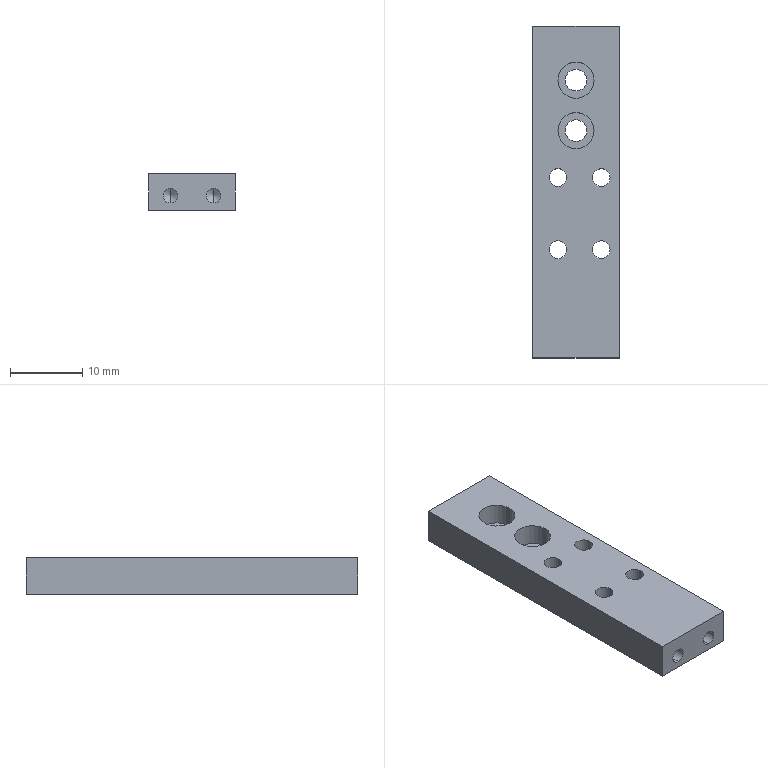Part | SolidWorks | features BaseBody 1 | 1 solid | 32 faces | box 12 x 46 x 5 mm | volume 2467 mm3 | cylinder 20 | plane 8 | cone 4 | commonest cylinder face diameters 2.459 x8 2.013 x4 3 x4 5 x4
STEP:
#1=CARTESIAN_POINT('',(2.595,24.168,0.));
#2=VERTEX_POINT('',#1);
#3=CARTESIAN_POINT('',(-0.4046,24.168,0.));
#4=VERTEX_POINT('',#3);
#5=CARTESIAN_POINT('',(1.095,24.168,0.));
#6=DIRECTION('',(0.,0.,-1.));
#7=DIRECTION('',(1.,0.,0.));
#8=AXIS2_PLACEMENT_3D('',#5,#6,#7);
#9=CIRCLE('',#8,1.5);
#10=EDGE_CURVE('',#2,#4,#9,.T.);
#11=ORIENTED_EDGE('',*,*,#10,.T.);
#12=CARTESIAN_POINT('',(-0.4046,24.168,2.));
#13=VERTEX_POINT('',#12);
#14=CARTESIAN_POINT('',(-0.4046,24.168,-42.802));
#15=DIRECTION('',(0.,0.,1.));
#16=VECTOR('',#15,1000.);
#17=LINE('',#14,#16);
#18=EDGE_CURVE('',#4,#13,#17,.T.);
#19=ORIENTED_EDGE('',*,*,#18,.T.);
#20=CARTESIAN_POINT('',(2.595,24.168,2.));
#21=VERTEX_POINT('',#20);
#22=CARTESIAN_POINT('',(1.095,24.168,2.));
#23=DIRECTION('',(0.,0.,-1.));
#24=DIRECTION('',(1.,0.,0.));
#25=AXIS2_PLACEMENT_3D('',#22,#23,#24);
#26=CIRCLE('',#25,1.5);
#27=EDGE_CURVE('',#21,#13,#26,.T.);
#28=ORIENTED_EDGE('',*,*,#27,.F.);
#29=CARTESIAN_POINT('',(2.595,24.168,-42.802));
#30=DIRECTION('',(0.,0.,1.));
#31=VECTOR('',#30,1000.);
#32=LINE('',#29,#31);
#33=EDGE_CURVE('',#2,#21,#32,.T.);
#34=ORIENTED_EDGE('',*,*,#33,.F.);
#35=EDGE_LOOP('',(#11,#19,#28,#34));
#36=FACE_OUTER_BOUND('',#35,.T.);
#37=CARTESIAN_POINT('',(1.095,24.168,-42.802));
#38=DIRECTION('',(0.,0.,1.));
#39=DIRECTION('',(1.,0.,0.));
#40=AXIS2_PLACEMENT_3D('',#37,#38,#39);
#41=CYLINDRICAL_SURFACE('',#40,1.5);
#42=ADVANCED_FACE('',(#36),#41,.F.);
#43=CARTESIAN_POINT('',(2.595,31.168,0.));
#44=VERTEX_POINT('',#43);
#45=CARTESIAN_POINT('',(-0.4046,31.168,0.));
#46=VERTEX_POINT('',#45);
#47=CARTESIAN_POINT('',(1.095,31.168,0.));
#48=DIRECTION('',(0.,0.,-1.));
#49=DIRECTION('',(1.,0.,0.));
#50=AXIS2_PLACEMENT_3D('',#47,#48,#49);
#51=CIRCLE('',#50,1.5);
#52=EDGE_CURVE('',#44,#46,#51,.T.);
#53=ORIENTED_EDGE('',*,*,#52,.T.);
#54=CARTESIAN_POINT('',(-0.4046,31.168,2.));
#55=VERTEX_POINT('',#54);
#56=CARTESIAN_POINT('',(-0.4046,31.168,-42.802));
#57=DIRECTION('',(0.,0.,1.));
#58=VECTOR('',#57,1000.);
#59=LINE('',#56,#58);
#60=EDGE_CURVE('',#46,#55,#59,.T.);
#61=ORIENTED_EDGE('',*,*,#60,.T.);
#62=CARTESIAN_POINT('',(2.595,31.168,2.));
#63=VERTEX_POINT('',#62);
#64=CARTESIAN_POINT('',(1.095,31.168,2.));
#65=DIRECTION('',(0.,0.,-1.));
#66=DIRECTION('',(1.,0.,0.));
#67=AXIS2_PLACEMENT_3D('',#64,#65,#66);
#68=CIRCLE('',#67,1.5);
#69=EDGE_CURVE('',#63,#55,#68,.T.);
#70=ORIENTED_EDGE('',*,*,#69,.F.);
#71=CARTESIAN_POINT('',(2.595,31.168,-42.802));
#72=DIRECTION('',(0.,0.,1.));
#73=VECTOR('',#72,1000.);
#74=LINE('',#71,#73);
#75=EDGE_CURVE('',#44,#63,#74,.T.);
#76=ORIENTED_EDGE('',*,*,#75,.F.);
#77=EDGE_LOOP('',(#53,#61,#70,#76));
#78=FACE_OUTER_BOUND('',#77,.T.);
#79=CARTESIAN_POINT('',(1.095,31.168,-42.802));
#80=DIRECTION('',(0.,0.,1.));
#81=DIRECTION('',(1.,0.,0.));
#82=AXIS2_PLACEMENT_3D('',#79,#80,#81);
#83=CYLINDRICAL_SURFACE('',#82,1.5);
#84=ADVANCED_FACE('',(#78),#83,.F.);
#85=CARTESIAN_POINT('',(-0.1751,7.668,0.));
#86=VERTEX_POINT('',#85);
#87=CARTESIAN_POINT('',(-2.634,7.668,0.));
#88=VERTEX_POINT('',#87);
#89=CARTESIAN_POINT('',(-1.405,7.668,0.));
#90=DIRECTION('',(0.,0.,-1.));
#91=DIRECTION('',(1.,0.,0.));
#92=AXIS2_PLACEMENT_3D('',#89,#90,#91);
#93=CIRCLE('',#92,1.23);
#94=EDGE_CURVE('',#86,#88,#93,.T.);
#95=ORIENTED_EDGE('',*,*,#94,.T.);
#96=CARTESIAN_POINT('',(-2.634,7.668,5.));
#97=VERTEX_POINT('',#96);
#98=CARTESIAN_POINT('',(-2.634,7.668,-42.802));
#99=DIRECTION('',(0.,0.,1.));
#100=VECTOR('',#99,1000.);
#101=LINE('',#98,#100);
#102=EDGE_CURVE('',#88,#97,#101,.T.);
#103=ORIENTED_EDGE('',*,*,#102,.T.);
#104=CARTESIAN_POINT('',(-0.1751,7.668,5.));
#105=VERTEX_POINT('',#104);
#106=CARTESIAN_POINT('',(-1.405,7.668,5.));
#107=DIRECTION('',(0.,0.,-1.));
#108=DIRECTION('',(1.,0.,0.));
#109=AXIS2_PLACEMENT_3D('',#106,#107,#108);
#110=CIRCLE('',#109,1.23);
#111=EDGE_CURVE('',#105,#97,#110,.T.);
#112=ORIENTED_EDGE('',*,*,#111,.F.);
#113=CARTESIAN_POINT('',(-0.1751,7.668,-42.802));
#114=DIRECTION('',(0.,0.,1.));
#115=VECTOR('',#114,1000.);
#116=LINE('',#113,#115);
#117=EDGE_CURVE('',#86,#105,#116,.T.);
#118=ORIENTED_EDGE('',*,*,#117,.F.);
#119=EDGE_LOOP('',(#95,#103,#112,#118));
#120=FACE_OUTER_BOUND('',#119,.T.);
#121=CARTESIAN_POINT('',(-1.405,7.668,-42.802));
#122=DIRECTION('',(0.,0.,1.));
#123=DIRECTION('',(1.,0.,0.));
#124=AXIS2_PLACEMENT_3D('',#121,#122,#123);
#125=CYLINDRICAL_SURFACE('',#124,1.23);
#126=ADVANCED_FACE('',(#120),#125,.F.);
#127=CARTESIAN_POINT('',(-0.1751,17.668,0.));
#128=VERTEX_POINT('',#127);
#129=CARTESIAN_POINT('',(-2.634,17.668,0.));
#130=VERTEX_POINT('',#129);
#131=CARTESIAN_POINT('',(-1.405,17.668,0.));
#132=DIRECTION('',(0.,0.,-1.));
#133=DIRECTION('',(1.,0.,0.));
#134=AXIS2_PLACEMENT_3D('',#131,#132,#133);
#135=CIRCLE('',#134,1.23);
#136=EDGE_CURVE('',#128,#130,#135,.T.);
#137=ORIENTED_EDGE('',*,*,#136,.T.);
#138=CARTESIAN_POINT('',(-2.634,17.668,5.));
#139=VERTEX_POINT('',#138);
#140=CARTESIAN_POINT('',(-2.634,17.668,-42.802));
#141=DIRECTION('',(0.,0.,1.));
#142=VECTOR('',#141,1000.);
#143=LINE('',#140,#142);
#144=EDGE_CURVE('',#130,#139,#143,.T.);
#145=ORIENTED_EDGE('',*,*,#144,.T.);
#146=CARTESIAN_POINT('',(-0.1751,17.668,5.));
#147=VERTEX_POINT('',#146);
#148=CARTESIAN_POINT('',(-1.405,17.668,5.));
#149=DIRECTION('',(0.,0.,-1.));
#150=DIRECTION('',(1.,0.,0.));
#151=AXIS2_PLACEMENT_3D('',#148,#149,#150);
#152=CIRCLE('',#151,1.23);
#153=EDGE_CURVE('',#147,#139,#152,.T.);
#154=ORIENTED_EDGE('',*,*,#153,.F.);
#155=CARTESIAN_POINT('',(-0.1751,17.668,-42.802));
#156=DIRECTION('',(0.,0.,1.));
#157=VECTOR('',#156,1000.);
#158=LINE('',#155,#157);
#159=EDGE_CURVE('',#128,#147,#158,.T.);
#160=ORIENTED_EDGE('',*,*,#159,.F.);
#161=EDGE_LOOP('',(#137,#145,#154,#160));
#162=FACE_OUTER_BOUND('',#161,.T.);
#163=CARTESIAN_POINT('',(-1.405,17.668,-42.802));
#164=DIRECTION('',(0.,0.,1.));
#165=DIRECTION('',(1.,0.,0.));
#166=AXIS2_PLACEMENT_3D('',#163,#164,#165);
#167=CYLINDRICAL_SURFACE('',#166,1.23);
#168=ADVANCED_FACE('',(#162),#167,.F.);
#169=CARTESIAN_POINT('',(5.825,17.668,0.));
#170=VERTEX_POINT('',#169);
#171=CARTESIAN_POINT('',(3.366,17.668,0.));
#172=VERTEX_POINT('',#171);
#173=CARTESIAN_POINT('',(4.595,17.668,0.));
#174=DIRECTION('',(0.,0.,-1.));
#175=DIRECTION('',(1.,0.,0.));
#176=AXIS2_PLACEMENT_3D('',#173,#174,#175);
#177=CIRCLE('',#176,1.229);
#178=EDGE_CURVE('',#170,#172,#177,.T.);
#179=ORIENTED_EDGE('',*,*,#178,.T.);
#180=CARTESIAN_POINT('',(3.366,17.668,5.));
#181=VERTEX_POINT('',#180);
#182=CARTESIAN_POINT('',(3.366,17.668,-42.802));
#183=DIRECTION('',(0.,0.,1.));
#184=VECTOR('',#183,1000.);
#185=LINE('',#182,#184);
#186=EDGE_CURVE('',#172,#181,#185,.T.);
#187=ORIENTED_EDGE('',*,*,#186,.T.);
#188=CARTESIAN_POINT('',(5.825,17.668,5.));
#189=VERTEX_POINT('',#188);
#190=CARTESIAN_POINT('',(4.595,17.668,5.));
#191=DIRECTION('',(0.,0.,-1.));
#192=DIRECTION('',(1.,0.,0.));
#193=AXIS2_PLACEMENT_3D('',#190,#191,#192);
#194=CIRCLE('',#193,1.229);
#195=EDGE_CURVE('',#189,#181,#194,.T.);
#196=ORIENTED_EDGE('',*,*,#195,.F.);
#197=CARTESIAN_POINT('',(5.825,17.668,-42.802));
#198=DIRECTION('',(0.,0.,1.));
#199=VECTOR('',#198,1000.);
#200=LINE('',#197,#199);
#201=EDGE_CURVE('',#170,#189,#200,.T.);
#202=ORIENTED_EDGE('',*,*,#201,.F.);
#203=EDGE_LOOP('',(#179,#187,#196,#202));
#204=FACE_OUTER_BOUND('',#203,.T.);
#205=CARTESIAN_POINT('',(4.595,17.668,-42.802));
#206=DIRECTION('',(0.,0.,1.));
#207=DIRECTION('',(1.,0.,0.));
#208=AXIS2_PLACEMENT_3D('',#205,#206,#207);
#209=CYLINDRICAL_SURFACE('',#208,1.229);
#210=ADVANCED_FACE('',(#204),#209,.F.);
#211=CARTESIAN_POINT('',(5.825,7.668,0.));
#212=VERTEX_POINT('',#211);
#213=CARTESIAN_POINT('',(3.366,7.668,0.));
#214=VERTEX_POINT('',#213);
#215=CARTESIAN_POINT('',(4.595,7.668,0.));
#216=DIRECTION('',(0.,0.,-1.));
#217=DIRECTION('',(1.,0.,0.));
#218=AXIS2_PLACEMENT_3D('',#215,#216,#217);
#219=CIRCLE('',#218,1.23);
#220=EDGE_CURVE('',#212,#214,#219,.T.);
#221=ORIENTED_EDGE('',*,*,#220,.T.);
#222=CARTESIAN_POINT('',(3.366,7.668,5.));
#223=VERTEX_POINT('',#222);
#224=CARTESIAN_POINT('',(3.366,7.668,-42.802));
#225=DIRECTION('',(0.,0.,1.));
#226=VECTOR('',#225,1000.);
#227=LINE('',#224,#226);
#228=EDGE_CURVE('',#214,#223,#227,.T.);
#229=ORIENTED_EDGE('',*,*,#228,.T.);
#230=CARTESIAN_POINT('',(5.825,7.668,5.));
#231=VERTEX_POINT('',#230);
#232=CARTESIAN_POINT('',(4.595,7.668,5.));
#233=DIRECTION('',(0.,0.,-1.));
#234=DIRECTION('',(1.,0.,0.));
#235=AXIS2_PLACEMENT_3D('',#232,#233,#234);
#236=CIRCLE('',#235,1.23);
#237=EDGE_CURVE('',#231,#223,#236,.T.);
#238=ORIENTED_EDGE('',*,*,#237,.F.);
#239=CARTESIAN_POINT('',(5.825,7.668,-42.802));
#240=DIRECTION('',(0.,0.,1.));
#241=VECTOR('',#240,1000.);
#242=LINE('',#239,#241);
#243=EDGE_CURVE('',#212,#231,#242,.T.);
#244=ORIENTED_EDGE('',*,*,#243,.F.);
#245=EDGE_LOOP('',(#221,#229,#238,#244));
#246=FACE_OUTER_BOUND('',#245,.T.);
#247=CARTESIAN_POINT('',(4.595,7.668,-42.802));
#248=DIRECTION('',(0.,0.,1.));
#249=DIRECTION('',(1.,0.,0.));
#250=AXIS2_PLACEMENT_3D('',#247,#248,#249);
#251=CYLINDRICAL_SURFACE('',#250,1.23);
#252=ADVANCED_FACE('',(#246),#251,.F.);
#253=CARTESIAN_POINT('',(-1.905,0.6681,3.006));
#254=VERTEX_POINT('',#253);
#255=CARTESIAN_POINT('',(-1.905,0.6681,0.9935));
#256=VERTEX_POINT('',#255);
#257=CARTESIAN_POINT('',(-1.905,0.6681,2.));
#258=DIRECTION('',(0.,-1.,0.));
#259=DIRECTION('',(0.,0.,-1.));
#260=AXIS2_PLACEMENT_3D('',#257,#258,#259);
#261=CIRCLE('',#260,1.006);
#262=EDGE_CURVE('',#254,#256,#261,.T.);
#263=ORIENTED_EDGE('',*,*,#262,.F.);
#264=CARTESIAN_POINT('',(-1.905,-7.332,3.006));
#265=VERTEX_POINT('',#264);
#266=CARTESIAN_POINT('',(-1.905,-3.332,3.006));
#267=DIRECTION('',(0.,-1.,0.));
#268=VECTOR('',#267,1000.);
#269=LINE('',#266,#268);
#270=EDGE_CURVE('',#254,#265,#269,.T.);
#271=ORIENTED_EDGE('',*,*,#270,.T.);
#272=CARTESIAN_POINT('',(-1.905,-7.332,0.9935));
#273=VERTEX_POINT('',#272);
#274=CARTESIAN_POINT('',(-1.905,-7.332,2.));
#275=DIRECTION('',(0.,1.,0.));
#276=DIRECTION('',(0.,0.,-1.));
#277=AXIS2_PLACEMENT_3D('',#274,#275,#276);
#278=CIRCLE('',#277,1.006);
#279=EDGE_CURVE('',#273,#265,#278,.T.);
#280=ORIENTED_EDGE('',*,*,#279,.F.);
#281=CARTESIAN_POINT('',(-1.905,-3.332,0.9935));
#282=DIRECTION('',(0.,-1.,0.));
#283=VECTOR('',#282,1000.);
#284=LINE('',#281,#283);
#285=EDGE_CURVE('',#256,#273,#284,.T.);
#286=ORIENTED_EDGE('',*,*,#285,.F.);
#287=EDGE_LOOP('',(#263,#271,#280,#286));
#288=FACE_OUTER_BOUND('',#287,.T.);
#289=CARTESIAN_POINT('',(-1.905,-3.332,2.));
#290=DIRECTION('',(0.,-1.,0.));
#291=DIRECTION('',(0.,0.,-1.));
#292=AXIS2_PLACEMENT_3D('',#289,#290,#291);
#293=CYLINDRICAL_SURFACE('',#292,1.006);
#294=ADVANCED_FACE('',(#288),#293,.F.);
#295=CARTESIAN_POINT('',(4.095,0.6681,3.006));
#296=VERTEX_POINT('',#295);
#297=CARTESIAN_POINT('',(4.095,0.6681,0.9935));
#298=VERTEX_POINT('',#297);
#299=CARTESIAN_POINT('',(4.095,0.6681,2.));
#300=DIRECTION('',(0.,-1.,0.));
#301=DIRECTION('',(0.,0.,-1.));
#302=AXIS2_PLACEMENT_3D('',#299,#300,#301);
#303=CIRCLE('',#302,1.006);
#304=EDGE_CURVE('',#296,#298,#303,.T.);
#305=ORIENTED_EDGE('',*,*,#304,.F.);
#306=CARTESIAN_POINT('',(4.095,-7.332,3.006));
#307=VERTEX_POINT('',#306);
#308=CARTESIAN_POINT('',(4.095,-3.332,3.006));
#309=DIRECTION('',(0.,-1.,0.));
#310=VECTOR('',#309,1000.);
#311=LINE('',#308,#310);
#312=EDGE_CURVE('',#296,#307,#311,.T.);
#313=ORIENTED_EDGE('',*,*,#312,.T.);
#314=CARTESIAN_POINT('',(4.095,-7.332,0.9935));
#315=VERTEX_POINT('',#314);
#316=CARTESIAN_POINT('',(4.095,-7.332,2.));
#317=DIRECTION('',(0.,1.,0.));
#318=DIRECTION('',(0.,0.,-1.));
#319=AXIS2_PLACEMENT_3D('',#316,#317,#318);
#320=CIRCLE('',#319,1.006);
#321=EDGE_CURVE('',#315,#307,#320,.T.);
#322=ORIENTED_EDGE('',*,*,#321,.F.);
#323=CARTESIAN_POINT('',(4.095,-3.332,0.9935));
#324=DIRECTION('',(0.,-1.,0.));
#325=VECTOR('',#324,1000.);
#326=LINE('',#323,#325);
#327=EDGE_CURVE('',#298,#315,#326,.T.);
#328=ORIENTED_EDGE('',*,*,#327,.F.);
#329=EDGE_LOOP('',(#305,#313,#322,#328));
#330=FACE_OUTER_BOUND('',#329,.T.);
#331=CARTESIAN_POINT('',(4.095,-3.332,2.));
#332=DIRECTION('',(0.,-1.,0.));
#333=DIRECTION('',(0.,0.,-1.));
#334=AXIS2_PLACEMENT_3D('',#331,#332,#333);
#335=CYLINDRICAL_SURFACE('',#334,1.006);
#336=ADVANCED_FACE('',(#330),#335,.F.);
#337=CARTESIAN_POINT('',(-1.405,24.168,2.));
#338=VERTEX_POINT('',#337);
#339=CARTESIAN_POINT('',(3.595,24.168,2.));
#340=VERTEX_POINT('',#339);
#341=CARTESIAN_POINT('',(1.095,24.168,2.));
#342=DIRECTION('',(0.,0.,1.));
#343=DIRECTION('',(1.,0.,0.));
#344=AXIS2_PLACEMENT_3D('',#341,#342,#343);
#345=CIRCLE('',#344,2.5);
#346=EDGE_CURVE('',#338,#340,#345,.T.);
#347=ORIENTED_EDGE('',*,*,#346,.F.);
#348=CARTESIAN_POINT('',(-1.405,24.168,5.));
#349=VERTEX_POINT('',#348);
#350=CARTESIAN_POINT('',(-1.405,24.168,3.5));
#351=DIRECTION('',(0.,0.,1.));
#352=VECTOR('',#351,1000.);
#353=LINE('',#350,#352);
#354=EDGE_CURVE('',#338,#349,#353,.T.);
#355=ORIENTED_EDGE('',*,*,#354,.T.);
#356=CARTESIAN_POINT('',(3.595,24.168,5.));
#357=VERTEX_POINT('',#356);
#358=CARTESIAN_POINT('',(1.095,24.168,5.));
#359=DIRECTION('',(0.,0.,-1.));
#360=DIRECTION('',(1.,0.,0.));
#361=AXIS2_PLACEMENT_3D('',#358,#359,#360);
#362=CIRCLE('',#361,2.5);
#363=EDGE_CURVE('',#357,#349,#362,.T.);
#364=ORIENTED_EDGE('',*,*,#363,.F.);
#365=CARTESIAN_POINT('',(3.595,24.168,3.5));
#366=DIRECTION('',(0.,0.,1.));
#367=VECTOR('',#366,1000.);
#368=LINE('',#365,#367);
#369=EDGE_CURVE('',#340,#357,#368,.T.);
#370=ORIENTED_EDGE('',*,*,#369,.F.);
#371=EDGE_LOOP('',(#347,#355,#364,#370));
#372=FACE_OUTER_BOUND('',#371,.T.);
#373=CARTESIAN_POINT('',(1.095,24.168,3.5));
#374=DIRECTION('',(0.,0.,1.));
#375=DIRECTION('',(1.,0.,0.));
#376=AXIS2_PLACEMENT_3D('',#373,#374,#375);
#377=CYLINDRICAL_SURFACE('',#376,2.5);
#378=ADVANCED_FACE('',(#372),#377,.F.);
#379=CARTESIAN_POINT('',(-1.405,31.168,2.));
#380=VERTEX_POINT('',#379);
#381=CARTESIAN_POINT('',(3.595,31.168,2.));
#382=VERTEX_POINT('',#381);
#383=CARTESIAN_POINT('',(1.095,31.168,2.));
#384=DIRECTION('',(0.,0.,1.));
#385=DIRECTION('',(1.,0.,0.));
#386=AXIS2_PLACEMENT_3D('',#383,#384,#385);
#387=CIRCLE('',#386,2.5);
#388=EDGE_CURVE('',#380,#382,#387,.T.);
#389=ORIENTED_EDGE('',*,*,#388,.F.);
#390=CARTESIAN_POINT('',(-1.405,31.168,5.));
#391=VERTEX_POINT('',#390);
#392=CARTESIAN_POINT('',(-1.405,31.168,3.5));
#393=DIRECTION('',(0.,0.,1.));
#394=VECTOR('',#393,1000.);
#395=LINE('',#392,#394);
#396=EDGE_CURVE('',#380,#391,#395,.T.);
#397=ORIENTED_EDGE('',*,*,#396,.T.);
#398=CARTESIAN_POINT('',(3.595,31.168,5.));
#399=VERTEX_POINT('',#398);
#400=CARTESIAN_POINT('',(1.095,31.168,5.));
#401=DIRECTION('',(0.,0.,-1.));
#402=DIRECTION('',(1.,0.,0.));
#403=AXIS2_PLACEMENT_3D('',#400,#401,#402);
#404=CIRCLE('',#403,2.5);
#405=EDGE_CURVE('',#399,#391,#404,.T.);
#406=ORIENTED_EDGE('',*,*,#405,.F.);
#407=CARTESIAN_POINT('',(3.595,31.168,3.5));
#408=DIRECTION('',(0.,0.,1.));
#409=VECTOR('',#408,1000.);
#410=LINE('',#407,#409);
#411=EDGE_CURVE('',#382,#399,#410,.T.);
#412=ORIENTED_EDGE('',*,*,#411,.F.);
#413=EDGE_LOOP('',(#389,#397,#406,#412));
#414=FACE_OUTER_BOUND('',#413,.T.);
#415=CARTESIAN_POINT('',(1.095,31.168,3.5));
#416=DIRECTION('',(0.,0.,1.));
#417=DIRECTION('',(1.,0.,0.));
#418=AXIS2_PLACEMENT_3D('',#415,#416,#417);
#419=CYLINDRICAL_SURFACE('',#418,2.5);
#420=ADVANCED_FACE('',(#414),#419,.F.);
#421=CARTESIAN_POINT('',(-1.905,1.273,2.));
#422=VERTEX_POINT('',#421);
#423=CARTESIAN_POINT('',(-1.905,0.6681,0.9935));
#424=DIRECTION('',(0.,-0.515,-0.8572));
#425=VECTOR('',#424,1000.);
#426=LINE('',#423,#425);
#427=EDGE_CURVE('',#422,#256,#426,.T.);
#428=ORIENTED_EDGE('',*,*,#427,.F.);
#429=CARTESIAN_POINT('',(-1.905,0.6681,3.006));
#430=DIRECTION('',(0.,-0.515,0.8572));
#431=VECTOR('',#430,1000.);
#432=LINE('',#429,#431);
#433=EDGE_CURVE('',#422,#254,#432,.T.);
#434=ORIENTED_EDGE('',*,*,#433,.T.);
#435=ORIENTED_EDGE('',*,*,#262,.T.);
#436=EDGE_LOOP('',(#428,#434,#435));
#437=FACE_OUTER_BOUND('',#436,.T.);
#438=CARTESIAN_POINT('',(-1.905,0.6681,2.));
#439=DIRECTION('',(0.,-1.,0.));
#440=DIRECTION('',(0.,0.,-1.));
#441=AXIS2_PLACEMENT_3D('',#438,#439,#440);
#442=CONICAL_SURFACE('',#441,1.006,1.03);
#443=ADVANCED_FACE('',(#437),#442,.F.);
#444=CARTESIAN_POINT('',(4.095,1.273,2.));
#445=VERTEX_POINT('',#444);
#446=CARTESIAN_POINT('',(4.095,0.6681,0.9935));
#447=DIRECTION('',(0.,-0.515,-0.8572));
#448=VECTOR('',#447,1000.);
#449=LINE('',#446,#448);
#450=EDGE_CURVE('',#445,#298,#449,.T.);
#451=ORIENTED_EDGE('',*,*,#450,.F.);
#452=CARTESIAN_POINT('',(4.095,0.6681,3.006));
#453=DIRECTION('',(0.,-0.515,0.8572));
#454=VECTOR('',#453,1000.);
#455=LINE('',#452,#454);
#456=EDGE_CURVE('',#445,#296,#455,.T.);
#457=ORIENTED_EDGE('',*,*,#456,.T.);
#458=ORIENTED_EDGE('',*,*,#304,.T.);
#459=EDGE_LOOP('',(#451,#457,#458));
#460=FACE_OUTER_BOUND('',#459,.T.);
#461=CARTESIAN_POINT('',(4.095,0.6681,2.));
#462=DIRECTION('',(0.,-1.,0.));
#463=DIRECTION('',(0.,0.,-1.));
#464=AXIS2_PLACEMENT_3D('',#461,#462,#463);
#465=CONICAL_SURFACE('',#464,1.006,1.03);
#466=ADVANCED_FACE('',(#460),#465,.F.);
#467=ORIENTED_EDGE('',*,*,#10,.F.);
#468=CARTESIAN_POINT('',(1.095,24.168,0.));
#469=DIRECTION('',(0.,0.,-1.));
#470=DIRECTION('',(1.,0.,0.));
#471=AXIS2_PLACEMENT_3D('',#468,#469,#470);
#472=CIRCLE('',#471,1.5);
#473=EDGE_CURVE('',#4,#2,#472,.T.);
#474=ORIENTED_EDGE('',*,*,#473,.F.);
#475=EDGE_LOOP('',(#467,#474));
#476=FACE_BOUND('',#475,.T.);
#477=ORIENTED_EDGE('',*,*,#52,.F.);
#478=CARTESIAN_POINT('',(1.095,31.168,0.));
#479=DIRECTION('',(0.,0.,-1.));
#480=DIRECTION('',(1.,0.,0.));
#481=AXIS2_PLACEMENT_3D('',#478,#479,#480);
#482=CIRCLE('',#481,1.5);
#483=EDGE_CURVE('',#46,#44,#482,.T.);
#484=ORIENTED_EDGE('',*,*,#483,.F.);
#485=EDGE_LOOP('',(#477,#484));
#486=FACE_BOUND('',#485,.T.);
#487=ORIENTED_EDGE('',*,*,#94,.F.);
#488=CARTESIAN_POINT('',(-1.405,7.668,0.));
#489=DIRECTION('',(0.,0.,-1.));
#490=DIRECTION('',(1.,0.,0.));
#491=AXIS2_PLACEMENT_3D('',#488,#489,#490);
#492=CIRCLE('',#491,1.23);
#493=EDGE_CURVE('',#88,#86,#492,.T.);
#494=ORIENTED_EDGE('',*,*,#493,.F.);
#495=EDGE_LOOP('',(#487,#494));
#496=FACE_BOUND('',#495,.T.);
#497=ORIENTED_EDGE('',*,*,#136,.F.);
#498=CARTESIAN_POINT('',(-1.405,17.668,0.));
#499=DIRECTION('',(0.,0.,-1.));
#500=DIRECTION('',(1.,0.,0.));
#501=AXIS2_PLACEMENT_3D('',#498,#499,#500);
#502=CIRCLE('',#501,1.23);
#503=EDGE_CURVE('',#130,#128,#502,.T.);
#504=ORIENTED_EDGE('',*,*,#503,.F.);
#505=EDGE_LOOP('',(#497,#504));
#506=FACE_BOUND('',#505,.T.);
#507=ORIENTED_EDGE('',*,*,#178,.F.);
#508=CARTESIAN_POINT('',(4.595,17.668,0.));
#509=DIRECTION('',(0.,0.,-1.));
#510=DIRECTION('',(1.,0.,0.));
#511=AXIS2_PLACEMENT_3D('',#508,#509,#510);
#512=CIRCLE('',#511,1.229);
#513=EDGE_CURVE('',#172,#170,#512,.T.);
#514=ORIENTED_EDGE('',*,*,#513,.F.);
#515=EDGE_LOOP('',(#507,#514));
#516=FACE_BOUND('',#515,.T.);
#517=ORIENTED_EDGE('',*,*,#220,.F.);
#518=CARTESIAN_POINT('',(4.595,7.668,0.));
#519=DIRECTION('',(0.,0.,-1.));
#520=DIRECTION('',(1.,0.,0.));
#521=AXIS2_PLACEMENT_3D('',#518,#519,#520);
#522=CIRCLE('',#521,1.23);
#523=EDGE_CURVE('',#214,#212,#522,.T.);
#524=ORIENTED_EDGE('',*,*,#523,.F.);
#525=EDGE_LOOP('',(#517,#524));
#526=FACE_BOUND('',#525,.T.);
#527=CARTESIAN_POINT('',(-4.905,38.668,0.));
#528=VERTEX_POINT('',#527);
#529=CARTESIAN_POINT('',(-4.905,-7.332,0.));
#530=VERTEX_POINT('',#529);
#531=CARTESIAN_POINT('',(-4.905,15.668,0.));
#532=DIRECTION('',(0.,-1.,0.));
#533=VECTOR('',#532,1000.);
#534=LINE('',#531,#533);
#535=EDGE_CURVE('',#528,#530,#534,.T.);
#536=ORIENTED_EDGE('',*,*,#535,.F.);
#537=CARTESIAN_POINT('',(7.095,38.668,0.));
#538=VERTEX_POINT('',#537);
#539=CARTESIAN_POINT('',(1.095,38.668,0.));
#540=DIRECTION('',(-1.,0.,0.));
#541=VECTOR('',#540,1000.);
#542=LINE('',#539,#541);
#543=EDGE_CURVE('',#538,#528,#542,.T.);
#544=ORIENTED_EDGE('',*,*,#543,.F.);
#545=CARTESIAN_POINT('',(7.095,-7.332,0.));
#546=VERTEX_POINT('',#545);
#547=CARTESIAN_POINT('',(7.095,15.668,0.));
#548=DIRECTION('',(0.,1.,0.));
#549=VECTOR('',#548,1000.);
#550=LINE('',#547,#549);
#551=EDGE_CURVE('',#546,#538,#550,.T.);
#552=ORIENTED_EDGE('',*,*,#551,.F.);
#553=CARTESIAN_POINT('',(1.095,-7.332,0.));
#554=DIRECTION('',(1.,0.,0.));
#555=VECTOR('',#554,1000.);
#556=LINE('',#553,#555);
#557=EDGE_CURVE('',#530,#546,#556,.T.);
#558=ORIENTED_EDGE('',*,*,#557,.F.);
#559=EDGE_LOOP('',(#536,#544,#552,#558));
#560=FACE_OUTER_BOUND('',#559,.T.);
#561=CARTESIAN_POINT('',(1.095,15.668,0.));
#562=DIRECTION('',(0.,0.,1.));
#563=DIRECTION('',(1.,0.,0.));
#564=AXIS2_PLACEMENT_3D('',#561,#562,#563);
#565=PLANE('',#564);
#566=ADVANCED_FACE('',(#476,#486,#496,#506,#516,#526,#560),#565,.F.);
#567=ORIENTED_EDGE('',*,*,#18,.F.);
#568=ORIENTED_EDGE('',*,*,#473,.T.);
#569=ORIENTED_EDGE('',*,*,#33,.T.);
#570=CARTESIAN_POINT('',(1.095,24.168,2.));
#571=DIRECTION('',(0.,0.,-1.));
#572=DIRECTION('',(1.,0.,0.));
#573=AXIS2_PLACEMENT_3D('',#570,#571,#572);
#574=CIRCLE('',#573,1.5);
#575=EDGE_CURVE('',#13,#21,#574,.T.);
#576=ORIENTED_EDGE('',*,*,#575,.F.);
#577=EDGE_LOOP('',(#567,#568,#569,#576));
#578=FACE_OUTER_BOUND('',#577,.T.);
#579=CARTESIAN_POINT('',(1.095,24.168,-42.802));
#580=DIRECTION('',(0.,0.,1.));
#581=DIRECTION('',(1.,0.,0.));
#582=AXIS2_PLACEMENT_3D('',#579,#580,#581);
#583=CYLINDRICAL_SURFACE('',#582,1.5);
#584=ADVANCED_FACE('',(#578),#583,.F.);
#585=ORIENTED_EDGE('',*,*,#60,.F.);
#586=ORIENTED_EDGE('',*,*,#483,.T.);
#587=ORIENTED_EDGE('',*,*,#75,.T.);
#588=CARTESIAN_POINT('',(1.095,31.168,2.));
#589=DIRECTION('',(0.,0.,-1.));
#590=DIRECTION('',(1.,0.,0.));
#591=AXIS2_PLACEMENT_3D('',#588,#589,#590);
#592=CIRCLE('',#591,1.5);
#593=EDGE_CURVE('',#55,#63,#592,.T.);
#594=ORIENTED_EDGE('',*,*,#593,.F.);
#595=EDGE_LOOP('',(#585,#586,#587,#594));
#596=FACE_OUTER_BOUND('',#595,.T.);
#597=CARTESIAN_POINT('',(1.095,31.168,-42.802));
#598=DIRECTION('',(0.,0.,1.));
#599=DIRECTION('',(1.,0.,0.));
#600=AXIS2_PLACEMENT_3D('',#597,#598,#599);
#601=CYLINDRICAL_SURFACE('',#600,1.5);
#602=ADVANCED_FACE('',(#596),#601,.F.);
#603=ORIENTED_EDGE('',*,*,#102,.F.);
#604=ORIENTED_EDGE('',*,*,#493,.T.);
#605=ORIENTED_EDGE('',*,*,#117,.T.);
#606=CARTESIAN_POINT('',(-1.405,7.668,5.));
#607=DIRECTION('',(0.,0.,-1.));
#608=DIRECTION('',(1.,0.,0.));
#609=AXIS2_PLACEMENT_3D('',#606,#607,#608);
#610=CIRCLE('',#609,1.23);
#611=EDGE_CURVE('',#97,#105,#610,.T.);
#612=ORIENTED_EDGE('',*,*,#611,.F.);
#613=EDGE_LOOP('',(#603,#604,#605,#612));
#614=FACE_OUTER_BOUND('',#613,.T.);
#615=CARTESIAN_POINT('',(-1.405,7.668,-42.802));
#616=DIRECTION('',(0.,0.,1.));
#617=DIRECTION('',(1.,0.,0.));
#618=AXIS2_PLACEMENT_3D('',#615,#616,#617);
#619=CYLINDRICAL_SURFACE('',#618,1.23);
#620=ADVANCED_FACE('',(#614),#619,.F.);
#621=ORIENTED_EDGE('',*,*,#144,.F.);
#622=ORIENTED_EDGE('',*,*,#503,.T.);
#623=ORIENTED_EDGE('',*,*,#159,.T.);
#624=CARTESIAN_POINT('',(-1.405,17.668,5.));
#625=DIRECTION('',(0.,0.,-1.));
#626=DIRECTION('',(1.,0.,0.));
#627=AXIS2_PLACEMENT_3D('',#624,#625,#626);
#628=CIRCLE('',#627,1.23);
#629=EDGE_CURVE('',#139,#147,#628,.T.);
#630=ORIENTED_EDGE('',*,*,#629,.F.);
#631=EDGE_LOOP('',(#621,#622,#623,#630));
#632=FACE_OUTER_BOUND('',#631,.T.);
#633=CARTESIAN_POINT('',(-1.405,17.668,-42.802));
#634=DIRECTION('',(0.,0.,1.));
#635=DIRECTION('',(1.,0.,0.));
#636=AXIS2_PLACEMENT_3D('',#633,#634,#635);
#637=CYLINDRICAL_SURFACE('',#636,1.23);
#638=ADVANCED_FACE('',(#632),#637,.F.);
#639=ORIENTED_EDGE('',*,*,#186,.F.);
#640=ORIENTED_EDGE('',*,*,#513,.T.);
#641=ORIENTED_EDGE('',*,*,#201,.T.);
#642=CARTESIAN_POINT('',(4.595,17.668,5.));
#643=DIRECTION('',(0.,0.,-1.));
#644=DIRECTION('',(1.,0.,0.));
#645=AXIS2_PLACEMENT_3D('',#642,#643,#644);
#646=CIRCLE('',#645,1.229);
#647=EDGE_CURVE('',#181,#189,#646,.T.);
#648=ORIENTED_EDGE('',*,*,#647,.F.);
#649=EDGE_LOOP('',(#639,#640,#641,#648));
#650=FACE_OUTER_BOUND('',#649,.T.);
#651=CARTESIAN_POINT('',(4.595,17.668,-42.802));
#652=DIRECTION('',(0.,0.,1.));
#653=DIRECTION('',(1.,0.,0.));
#654=AXIS2_PLACEMENT_3D('',#651,#652,#653);
#655=CYLINDRICAL_SURFACE('',#654,1.229);
#656=ADVANCED_FACE('',(#650),#655,.F.);
#657=ORIENTED_EDGE('',*,*,#228,.F.);
#658=ORIENTED_EDGE('',*,*,#523,.T.);
#659=ORIENTED_EDGE('',*,*,#243,.T.);
#660=CARTESIAN_POINT('',(4.595,7.668,5.));
#661=DIRECTION('',(0.,0.,-1.));
#662=DIRECTION('',(1.,0.,0.));
#663=AXIS2_PLACEMENT_3D('',#660,#661,#662);
#664=CIRCLE('',#663,1.23);
#665=EDGE_CURVE('',#223,#231,#664,.T.);
#666=ORIENTED_EDGE('',*,*,#665,.F.);
#667=EDGE_LOOP('',(#657,#658,#659,#666));
#668=FACE_OUTER_BOUND('',#667,.T.);
#669=CARTESIAN_POINT('',(4.595,7.668,-42.802));
#670=DIRECTION('',(0.,0.,1.));
#671=DIRECTION('',(1.,0.,0.));
#672=AXIS2_PLACEMENT_3D('',#669,#670,#671);
#673=CYLINDRICAL_SURFACE('',#672,1.23);
#674=ADVANCED_FACE('',(#668),#673,.F.);
#675=ORIENTED_EDGE('',*,*,#279,.T.);
#676=CARTESIAN_POINT('',(-1.905,-7.332,2.));
#677=DIRECTION('',(0.,1.,0.));
#678=DIRECTION('',(0.,0.,-1.));
#679=AXIS2_PLACEMENT_3D('',#676,#677,#678);
#680=CIRCLE('',#679,1.006);
#681=EDGE_CURVE('',#265,#273,#680,.T.);
#682=ORIENTED_EDGE('',*,*,#681,.T.);
#683=EDGE_LOOP('',(#675,#682));
#684=FACE_BOUND('',#683,.T.);
#685=ORIENTED_EDGE('',*,*,#321,.T.);
#686=CARTESIAN_POINT('',(4.095,-7.332,2.));
#687=DIRECTION('',(0.,1.,0.));
#688=DIRECTION('',(0.,0.,-1.));
#689=AXIS2_PLACEMENT_3D('',#686,#687,#688);
#690=CIRCLE('',#689,1.006);
#691=EDGE_CURVE('',#307,#315,#690,.T.);
#692=ORIENTED_EDGE('',*,*,#691,.T.);
#693=EDGE_LOOP('',(#685,#692));
#694=FACE_BOUND('',#693,.T.);
#695=ORIENTED_EDGE('',*,*,#557,.T.);
#696=CARTESIAN_POINT('',(7.095,-7.332,5.));
#697=VERTEX_POINT('',#696);
#698=CARTESIAN_POINT('',(7.095,-7.332,0.));
#699=DIRECTION('',(0.,0.,1.));
#700=VECTOR('',#699,1000.);
#701=LINE('',#698,#700);
#702=EDGE_CURVE('',#546,#697,#701,.T.);
#703=ORIENTED_EDGE('',*,*,#702,.T.);
#704=CARTESIAN_POINT('',(-4.905,-7.332,5.));
#705=VERTEX_POINT('',#704);
#706=CARTESIAN_POINT('',(7.095,-7.332,5.));
#707=DIRECTION('',(-1.,0.,0.));
#708=VECTOR('',#707,1000.);
#709=LINE('',#706,#708);
#710=EDGE_CURVE('',#697,#705,#709,.T.);
#711=ORIENTED_EDGE('',*,*,#710,.T.);
#712=CARTESIAN_POINT('',(-4.905,-7.332,0.));
#713=DIRECTION('',(0.,0.,-1.));
#714=VECTOR('',#713,1000.);
#715=LINE('',#712,#714);
#716=EDGE_CURVE('',#705,#530,#715,.T.);
#717=ORIENTED_EDGE('',*,*,#716,.T.);
#718=EDGE_LOOP('',(#695,#703,#711,#717));
#719=FACE_OUTER_BOUND('',#718,.T.);
#720=CARTESIAN_POINT('',(7.095,-7.332,0.));
#721=DIRECTION('',(0.,-1.,0.));
#722=DIRECTION('',(0.,0.,-1.));
#723=AXIS2_PLACEMENT_3D('',#720,#721,#722);
#724=PLANE('',#723);
#725=ADVANCED_FACE('',(#684,#694,#719),#724,.T.);
#726=ORIENTED_EDGE('',*,*,#535,.T.);
#727=ORIENTED_EDGE('',*,*,#716,.F.);
#728=CARTESIAN_POINT('',(-4.905,38.668,5.));
#729=VERTEX_POINT('',#728);
#730=CARTESIAN_POINT('',(-4.905,-7.332,5.));
#731=DIRECTION('',(0.,1.,0.));
#732=VECTOR('',#731,1000.);
#733=LINE('',#730,#732);
#734=EDGE_CURVE('',#705,#729,#733,.T.);
#735=ORIENTED_EDGE('',*,*,#734,.T.);
#736=CARTESIAN_POINT('',(-4.905,38.668,0.));
#737=DIRECTION('',(0.,0.,-1.));
#738=VECTOR('',#737,1000.);
#739=LINE('',#736,#738);
#740=EDGE_CURVE('',#729,#528,#739,.T.);
#741=ORIENTED_EDGE('',*,*,#740,.T.);
#742=EDGE_LOOP('',(#726,#727,#735,#741));
#743=FACE_OUTER_BOUND('',#742,.T.);
#744=CARTESIAN_POINT('',(-4.905,-7.332,0.));
#745=DIRECTION('',(-1.,0.,0.));
#746=DIRECTION('',(0.,0.,1.));
#747=AXIS2_PLACEMENT_3D('',#744,#745,#746);
#748=PLANE('',#747);
#749=ADVANCED_FACE('',(#743),#748,.T.);
#750=ORIENTED_EDGE('',*,*,#543,.T.);
#751=ORIENTED_EDGE('',*,*,#740,.F.);
#752=CARTESIAN_POINT('',(7.095,38.668,5.));
#753=VERTEX_POINT('',#752);
#754=CARTESIAN_POINT('',(-4.905,38.668,5.));
#755=DIRECTION('',(1.,0.,0.));
#756=VECTOR('',#755,1000.);
#757=LINE('',#754,#756);
#758=EDGE_CURVE('',#729,#753,#757,.T.);
#759=ORIENTED_EDGE('',*,*,#758,.T.);
#760=CARTESIAN_POINT('',(7.095,38.668,0.));
#761=DIRECTION('',(0.,0.,-1.));
#762=VECTOR('',#761,1000.);
#763=LINE('',#760,#762);
#764=EDGE_CURVE('',#753,#538,#763,.T.);
#765=ORIENTED_EDGE('',*,*,#764,.T.);
#766=EDGE_LOOP('',(#750,#751,#759,#765));
#767=FACE_OUTER_BOUND('',#766,.T.);
#768=CARTESIAN_POINT('',(-4.905,38.668,0.));
#769=DIRECTION('',(0.,1.,0.));
#770=DIRECTION('',(0.,0.,1.));
#771=AXIS2_PLACEMENT_3D('',#768,#769,#770);
#772=PLANE('',#771);
#773=ADVANCED_FACE('',(#767),#772,.T.);
#774=ORIENTED_EDGE('',*,*,#551,.T.);
#775=ORIENTED_EDGE('',*,*,#764,.F.);
#776=CARTESIAN_POINT('',(7.095,38.668,5.));
#777=DIRECTION('',(0.,-1.,0.));
#778=VECTOR('',#777,1000.);
#779=LINE('',#776,#778);
#780=EDGE_CURVE('',#753,#697,#779,.T.);
#781=ORIENTED_EDGE('',*,*,#780,.T.);
#782=ORIENTED_EDGE('',*,*,#702,.F.);
#783=EDGE_LOOP('',(#774,#775,#781,#782));
#784=FACE_OUTER_BOUND('',#783,.T.);
#785=CARTESIAN_POINT('',(7.095,38.668,0.));
#786=DIRECTION('',(1.,0.,0.));
#787=DIRECTION('',(0.,0.,-1.));
#788=AXIS2_PLACEMENT_3D('',#785,#786,#787);
#789=PLANE('',#788);
#790=ADVANCED_FACE('',(#784),#789,.T.);
#791=ORIENTED_EDGE('',*,*,#27,.T.);
#792=ORIENTED_EDGE('',*,*,#575,.T.);
#793=EDGE_LOOP('',(#791,#792));
#794=FACE_BOUND('',#793,.T.);
#795=CARTESIAN_POINT('',(1.095,24.168,2.));
#796=DIRECTION('',(0.,0.,1.));
#797=DIRECTION('',(1.,0.,0.));
#798=AXIS2_PLACEMENT_3D('',#795,#796,#797);
#799=CIRCLE('',#798,2.5);
#800=EDGE_CURVE('',#340,#338,#799,.T.);
#801=ORIENTED_EDGE('',*,*,#800,.T.);
#802=ORIENTED_EDGE('',*,*,#346,.T.);
#803=EDGE_LOOP('',(#801,#802));
#804=FACE_OUTER_BOUND('',#803,.T.);
#805=CARTESIAN_POINT('',(1.095,24.168,2.));
#806=DIRECTION('',(0.,0.,1.));
#807=DIRECTION('',(1.,0.,0.));
#808=AXIS2_PLACEMENT_3D('',#805,#806,#807);
#809=PLANE('',#808);
#810=ADVANCED_FACE('',(#794,#804),#809,.T.);
#811=ORIENTED_EDGE('',*,*,#69,.T.);
#812=ORIENTED_EDGE('',*,*,#593,.T.);
#813=EDGE_LOOP('',(#811,#812));
#814=FACE_BOUND('',#813,.T.);
#815=CARTESIAN_POINT('',(1.095,31.168,2.));
#816=DIRECTION('',(0.,0.,1.));
#817=DIRECTION('',(1.,0.,0.));
#818=AXIS2_PLACEMENT_3D('',#815,#816,#817);
#819=CIRCLE('',#818,2.5);
#820=EDGE_CURVE('',#382,#380,#819,.T.);
#821=ORIENTED_EDGE('',*,*,#820,.T.);
#822=ORIENTED_EDGE('',*,*,#388,.T.);
#823=EDGE_LOOP('',(#821,#822));
#824=FACE_OUTER_BOUND('',#823,.T.);
#825=CARTESIAN_POINT('',(1.095,31.168,2.));
#826=DIRECTION('',(0.,0.,1.));
#827=DIRECTION('',(1.,0.,0.));
#828=AXIS2_PLACEMENT_3D('',#825,#826,#827);
#829=PLANE('',#828);
#830=ADVANCED_FACE('',(#814,#824),#829,.T.);
#831=ORIENTED_EDGE('',*,*,#363,.T.);
#832=CARTESIAN_POINT('',(1.095,24.168,5.));
#833=DIRECTION('',(0.,0.,-1.));
#834=DIRECTION('',(1.,0.,0.));
#835=AXIS2_PLACEMENT_3D('',#832,#833,#834);
#836=CIRCLE('',#835,2.5);
#837=EDGE_CURVE('',#349,#357,#836,.T.);
#838=ORIENTED_EDGE('',*,*,#837,.T.);
#839=EDGE_LOOP('',(#831,#838));
#840=FACE_BOUND('',#839,.T.);
#841=ORIENTED_EDGE('',*,*,#405,.T.);
#842=CARTESIAN_POINT('',(1.095,31.168,5.));
#843=DIRECTION('',(0.,0.,-1.));
#844=DIRECTION('',(1.,0.,0.));
#845=AXIS2_PLACEMENT_3D('',#842,#843,#844);
#846=CIRCLE('',#845,2.5);
#847=EDGE_CURVE('',#391,#399,#846,.T.);
#848=ORIENTED_EDGE('',*,*,#847,.T.);
#849=EDGE_LOOP('',(#841,#848));
#850=FACE_BOUND('',#849,.T.);
#851=ORIENTED_EDGE('',*,*,#111,.T.);
#852=ORIENTED_EDGE('',*,*,#611,.T.);
#853=EDGE_LOOP('',(#851,#852));
#854=FACE_BOUND('',#853,.T.);
#855=ORIENTED_EDGE('',*,*,#153,.T.);
#856=ORIENTED_EDGE('',*,*,#629,.T.);
#857=EDGE_LOOP('',(#855,#856));
#858=FACE_BOUND('',#857,.T.);
#859=ORIENTED_EDGE('',*,*,#195,.T.);
#860=ORIENTED_EDGE('',*,*,#647,.T.);
#861=EDGE_LOOP('',(#859,#860));
#862=FACE_BOUND('',#861,.T.);
#863=ORIENTED_EDGE('',*,*,#237,.T.);
#864=ORIENTED_EDGE('',*,*,#665,.T.);
#865=EDGE_LOOP('',(#863,#864));
#866=FACE_BOUND('',#865,.T.);
#867=ORIENTED_EDGE('',*,*,#780,.F.);
#868=ORIENTED_EDGE('',*,*,#758,.F.);
#869=ORIENTED_EDGE('',*,*,#734,.F.);
#870=ORIENTED_EDGE('',*,*,#710,.F.);
#871=EDGE_LOOP('',(#867,#868,#869,#870));
#872=FACE_OUTER_BOUND('',#871,.T.);
#873=CARTESIAN_POINT('',(1.095,15.668,5.));
#874=DIRECTION('',(0.,0.,1.));
#875=DIRECTION('',(1.,0.,0.));
#876=AXIS2_PLACEMENT_3D('',#873,#874,#875);
#877=PLANE('',#876);
#878=ADVANCED_FACE('',(#840,#850,#854,#858,#862,#866,#872),#877,.T.);
#879=ORIENTED_EDGE('',*,*,#270,.F.);
#880=CARTESIAN_POINT('',(-1.905,0.6681,2.));
#881=DIRECTION('',(0.,-1.,0.));
#882=DIRECTION('',(0.,0.,-1.));
#883=AXIS2_PLACEMENT_3D('',#880,#881,#882);
#884=CIRCLE('',#883,1.006);
#885=EDGE_CURVE('',#256,#254,#884,.T.);
#886=ORIENTED_EDGE('',*,*,#885,.F.);
#887=ORIENTED_EDGE('',*,*,#285,.T.);
#888=ORIENTED_EDGE('',*,*,#681,.F.);
#889=EDGE_LOOP('',(#879,#886,#887,#888));
#890=FACE_OUTER_BOUND('',#889,.T.);
#891=CARTESIAN_POINT('',(-1.905,-3.332,2.));
#892=DIRECTION('',(0.,-1.,0.));
#893=DIRECTION('',(0.,0.,-1.));
#894=AXIS2_PLACEMENT_3D('',#891,#892,#893);
#895=CYLINDRICAL_SURFACE('',#894,1.006);
#896=ADVANCED_FACE('',(#890),#895,.F.);
#897=ORIENTED_EDGE('',*,*,#312,.F.);
#898=CARTESIAN_POINT('',(4.095,0.6681,2.));
#899=DIRECTION('',(0.,-1.,0.));
#900=DIRECTION('',(0.,0.,-1.));
#901=AXIS2_PLACEMENT_3D('',#898,#899,#900);
#902=CIRCLE('',#901,1.006);
#903=EDGE_CURVE('',#298,#296,#902,.T.);
#904=ORIENTED_EDGE('',*,*,#903,.F.);
#905=ORIENTED_EDGE('',*,*,#327,.T.);
#906=ORIENTED_EDGE('',*,*,#691,.F.);
#907=EDGE_LOOP('',(#897,#904,#905,#906));
#908=FACE_OUTER_BOUND('',#907,.T.);
#909=CARTESIAN_POINT('',(4.095,-3.332,2.));
#910=DIRECTION('',(0.,-1.,0.));
#911=DIRECTION('',(0.,0.,-1.));
#912=AXIS2_PLACEMENT_3D('',#909,#910,#911);
#913=CYLINDRICAL_SURFACE('',#912,1.006);
#914=ADVANCED_FACE('',(#908),#913,.F.);
#915=ORIENTED_EDGE('',*,*,#354,.F.);
#916=ORIENTED_EDGE('',*,*,#800,.F.);
#917=ORIENTED_EDGE('',*,*,#369,.T.);
#918=ORIENTED_EDGE('',*,*,#837,.F.);
#919=EDGE_LOOP('',(#915,#916,#917,#918));
#920=FACE_OUTER_BOUND('',#919,.T.);
#921=CARTESIAN_POINT('',(1.095,24.168,3.5));
#922=DIRECTION('',(0.,0.,1.));
#923=DIRECTION('',(1.,0.,0.));
#924=AXIS2_PLACEMENT_3D('',#921,#922,#923);
#925=CYLINDRICAL_SURFACE('',#924,2.5);
#926=ADVANCED_FACE('',(#920),#925,.F.);
#927=ORIENTED_EDGE('',*,*,#396,.F.);
#928=ORIENTED_EDGE('',*,*,#820,.F.);
#929=ORIENTED_EDGE('',*,*,#411,.T.);
#930=ORIENTED_EDGE('',*,*,#847,.F.);
#931=EDGE_LOOP('',(#927,#928,#929,#930));
#932=FACE_OUTER_BOUND('',#931,.T.);
#933=CARTESIAN_POINT('',(1.095,31.168,3.5));
#934=DIRECTION('',(0.,0.,1.));
#935=DIRECTION('',(1.,0.,0.));
#936=AXIS2_PLACEMENT_3D('',#933,#934,#935);
#937=CYLINDRICAL_SURFACE('',#936,2.5);
#938=ADVANCED_FACE('',(#932),#937,.F.);
#939=ORIENTED_EDGE('',*,*,#433,.F.);
#940=ORIENTED_EDGE('',*,*,#427,.T.);
#941=ORIENTED_EDGE('',*,*,#885,.T.);
#942=EDGE_LOOP('',(#939,#940,#941));
#943=FACE_OUTER_BOUND('',#942,.T.);
#944=CARTESIAN_POINT('',(-1.905,0.6681,2.));
#945=DIRECTION('',(0.,-1.,0.));
#946=DIRECTION('',(0.,0.,-1.));
#947=AXIS2_PLACEMENT_3D('',#944,#945,#946);
#948=CONICAL_SURFACE('',#947,1.006,1.03);
#949=ADVANCED_FACE('',(#943),#948,.F.);
#950=ORIENTED_EDGE('',*,*,#456,.F.);
#951=ORIENTED_EDGE('',*,*,#450,.T.);
#952=ORIENTED_EDGE('',*,*,#903,.T.);
#953=EDGE_LOOP('',(#950,#951,#952));
#954=FACE_OUTER_BOUND('',#953,.T.);
#955=CARTESIAN_POINT('',(4.095,0.6681,2.));
#956=DIRECTION('',(0.,-1.,0.));
#957=DIRECTION('',(0.,0.,-1.));
#958=AXIS2_PLACEMENT_3D('',#955,#956,#957);
#959=CONICAL_SURFACE('',#958,1.006,1.03);
#960=ADVANCED_FACE('',(#954),#959,.F.);
#961=CLOSED_SHELL('',(#42,#84,#126,#168,#210,#252,#294,#336,#378,#420,#443,#466,#566,#584,#602,#620,#638,#656,#674,#725,#749,#773,#790,#810,#830,#878,#896,#914,#926,#938,#949,#960));
#962=MANIFOLD_SOLID_BREP('',#961);
#963=CARTESIAN_POINT('',(0.,0.,0.));
#964=DIRECTION('',(0.,0.,1.));
#965=DIRECTION('',(1.,0.,0.));
#966=AXIS2_PLACEMENT_3D('',#963,#964,#965);
#967=(LENGTH_UNIT()NAMED_UNIT(*)SI_UNIT(.MILLI.,.METRE.));
#968=UNCERTAINTY_MEASURE_WITH_UNIT(LENGTH_MEASURE(0.00001),#967,'','');
#969=(NAMED_UNIT(*)PLANE_ANGLE_UNIT()SI_UNIT($,.RADIAN.));
#970=(NAMED_UNIT(*)SI_UNIT($,.STERADIAN.)SOLID_ANGLE_UNIT());
#971=(GEOMETRIC_REPRESENTATION_CONTEXT(3)GLOBAL_UNCERTAINTY_ASSIGNED_CONTEXT((#968))GLOBAL_UNIT_ASSIGNED_CONTEXT((#967,#969,#970))REPRESENTATION_CONTEXT('',''));
#972=ADVANCED_BREP_SHAPE_REPRESENTATION('',(#962,#966),#971);